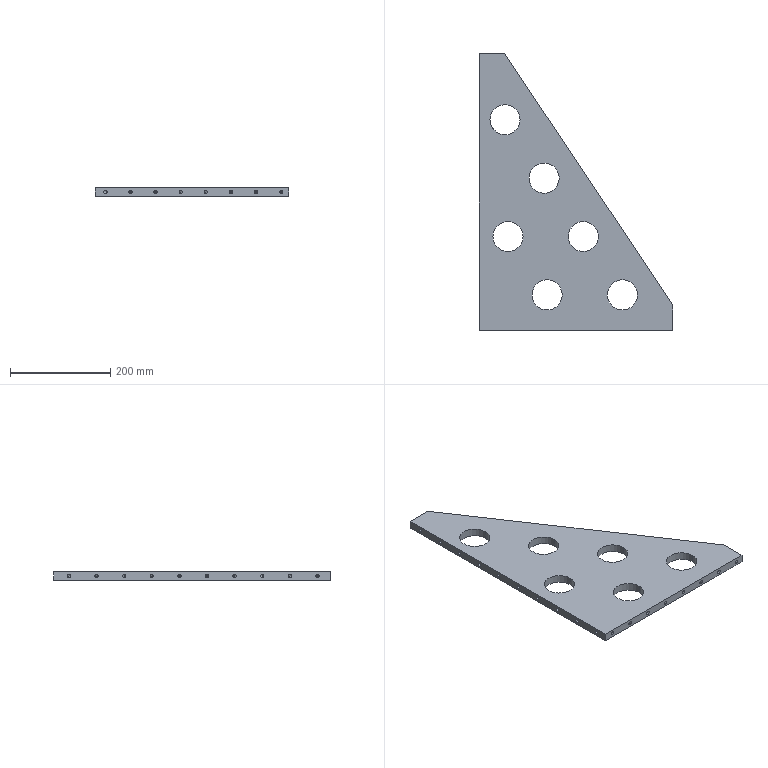Part | SolidWorks | features HoleWzd 2, LPattern 2, Extrusion 1, ICE 1 | 1 solid | 93 faces | box 385 x 550 x 16 mm | volume 1761626 mm3 | cylinder 48 | cone 38 | plane 7 | commonest cylinder face diameters 6.8 x36 60 x12